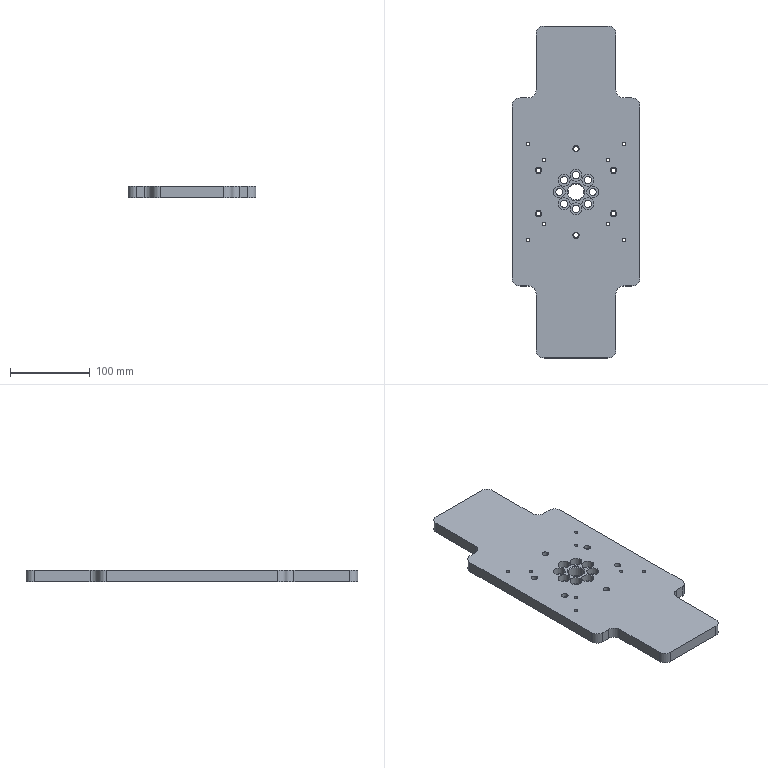Part | SolidWorks | features HoleWzd 3, CirPattern 2, ICE 2, Chamfer 1, Extrusion 1, Fillet 1, MirrorPattern 1 | 1 solid | 118 faces | box 160 x 415 x 14 mm | volume 752880 mm3 | cylinder 86 | plane 28 | cone 4 | commonest cylinder face diameters 4.2 x16 9 x16 15 x16 20 x14 6 x12 8 x12